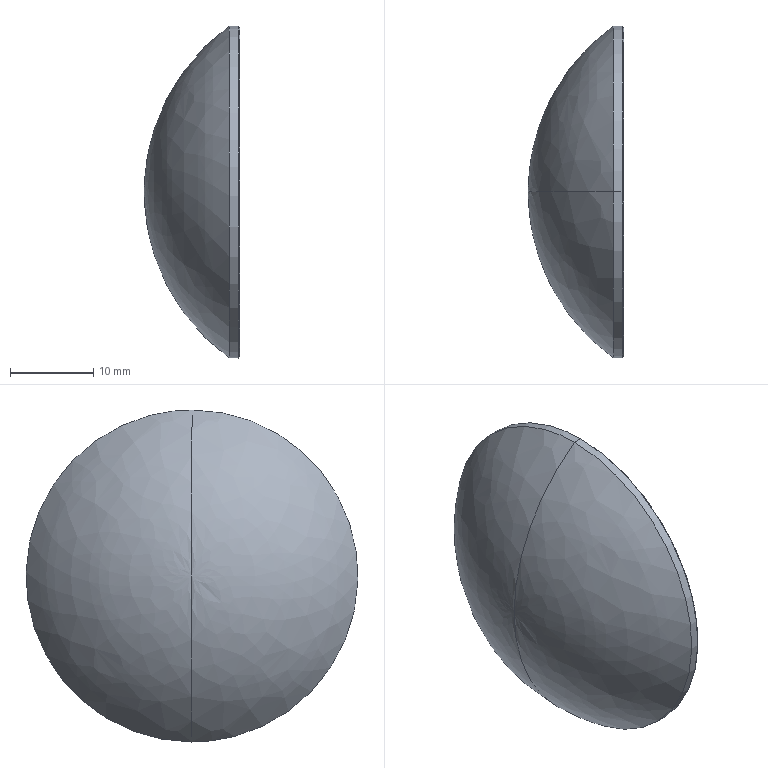Part | SolidWorks | features BaseBody 1 | 1 solid | 9 faces | box 11.433 x 39.8 x 39.8 mm | volume 7338 mm3 | spline 9
STEP:
#1=CARTESIAN_POINT('',(-56.988,0.,0.));
#2=VERTEX_POINT('',#1);
#3=CARTESIAN_POINT('',(-46.779,0.,19.9));
#4=VERTEX_POINT('',#3);
#5=CARTESIAN_POINT('',(-32.488,0.,0.));
#6=DIRECTION('',(0.,1.,0.));
#7=DIRECTION('',(-1.,0.,0.));
#8=AXIS2_PLACEMENT_3D('',#5,#6,#7);
#9=CIRCLE('',#8,24.5);
#10=EDGE_CURVE('',#2,#4,#9,.T.);
#11=ORIENTED_EDGE('',*,*,#10,.T.);
#12=CARTESIAN_POINT('',(-46.779,0.,-19.9));
#13=VERTEX_POINT('',#12);
#14=CARTESIAN_POINT('',(-46.779,0.,-19.9));
#15=CARTESIAN_POINT('',(-46.779,39.8,-19.9));
#16=CARTESIAN_POINT('',(-46.779,39.8,19.9));
#17=CARTESIAN_POINT('',(-46.779,0.,19.9));
#18=(BOUNDED_CURVE()B_SPLINE_CURVE(3,(#14,#15,#16,#17),.UNSPECIFIED.,.F.,.T.)B_SPLINE_CURVE_WITH_KNOTS((4,4),(0.,119.4),.UNSPECIFIED.)CURVE()GEOMETRIC_REPRESENTATION_ITEM()RATIONAL_B_SPLINE_CURVE((1.,0.3333,0.3333,1.))REPRESENTATION_ITEM(''));
#19=EDGE_CURVE('',#13,#4,#18,.T.);
#20=ORIENTED_EDGE('',*,*,#19,.F.);
#21=CARTESIAN_POINT('',(-32.488,0.,0.));
#22=DIRECTION('',(0.,-1.,0.));
#23=DIRECTION('',(-1.,0.,0.));
#24=AXIS2_PLACEMENT_3D('',#21,#22,#23);
#25=CIRCLE('',#24,24.5);
#26=EDGE_CURVE('',#2,#13,#25,.T.);
#27=ORIENTED_EDGE('',*,*,#26,.F.);
#28=EDGE_LOOP('',(#11,#20,#27));
#29=FACE_OUTER_BOUND('',#28,.T.);
#30=CARTESIAN_POINT('',(-56.988,0.,0.));
#31=CARTESIAN_POINT('',(-56.988,0.,0.));
#32=CARTESIAN_POINT('',(-56.988,0.,0.));
#33=CARTESIAN_POINT('',(-56.988,0.,0.));
#34=CARTESIAN_POINT('',(-56.988,0.,-8.047));
#35=CARTESIAN_POINT('',(-56.988,16.093,-8.047));
#36=CARTESIAN_POINT('',(-56.988,16.093,8.047));
#37=CARTESIAN_POINT('',(-56.988,0.,8.047));
#38=CARTESIAN_POINT('',(-53.315,0.,-15.206));
#39=CARTESIAN_POINT('',(-53.315,30.412,-15.206));
#40=CARTESIAN_POINT('',(-53.315,30.412,15.206));
#41=CARTESIAN_POINT('',(-53.315,0.,15.206));
#42=CARTESIAN_POINT('',(-46.779,0.,-19.9));
#43=CARTESIAN_POINT('',(-46.779,39.8,-19.9));
#44=CARTESIAN_POINT('',(-46.779,39.8,19.9));
#45=CARTESIAN_POINT('',(-46.779,0.,19.9));
#46=(BOUNDED_SURFACE()B_SPLINE_SURFACE(3,3,((#30,#31,#32,#33),(#34,#35,#36,#37),(#38,#39,#40,#41),(#42,#43,#44,#45)),.UNSPECIFIED.,.F.,.F.,.F.)B_SPLINE_SURFACE_WITH_KNOTS((4,4),(4,4),(0.,1.),(0.,1.),.UNSPECIFIED.)GEOMETRIC_REPRESENTATION_ITEM()RATIONAL_B_SPLINE_SURFACE(((1.,0.3333,0.3333,1.),(0.9265,0.3088,0.3088,0.9265),(0.9265,0.3088,0.3088,0.9265),(1.,0.3333,0.3333,1.)))REPRESENTATION_ITEM('')SURFACE());
#47=ADVANCED_FACE('',(#29),#46,.F.);
#48=ORIENTED_EDGE('',*,*,#26,.T.);
#49=CARTESIAN_POINT('',(-46.779,0.,19.9));
#50=CARTESIAN_POINT('',(-46.779,-39.8,19.9));
#51=CARTESIAN_POINT('',(-46.779,-39.8,-19.9));
#52=CARTESIAN_POINT('',(-46.779,0.,-19.9));
#53=(BOUNDED_CURVE()B_SPLINE_CURVE(3,(#49,#50,#51,#52),.UNSPECIFIED.,.F.,.F.)B_SPLINE_CURVE_WITH_KNOTS((4,4),(0.,119.4),.UNSPECIFIED.)CURVE()GEOMETRIC_REPRESENTATION_ITEM()RATIONAL_B_SPLINE_CURVE((1.,0.3333,0.3333,1.))REPRESENTATION_ITEM(''));
#54=EDGE_CURVE('',#4,#13,#53,.T.);
#55=ORIENTED_EDGE('',*,*,#54,.F.);
#56=ORIENTED_EDGE('',*,*,#10,.F.);
#57=EDGE_LOOP('',(#48,#55,#56));
#58=FACE_OUTER_BOUND('',#57,.T.);
#59=CARTESIAN_POINT('',(-56.988,0.,0.));
#60=CARTESIAN_POINT('',(-56.988,0.,0.));
#61=CARTESIAN_POINT('',(-56.988,0.,0.));
#62=CARTESIAN_POINT('',(-56.988,0.,0.));
#63=CARTESIAN_POINT('',(-56.988,0.,8.047));
#64=CARTESIAN_POINT('',(-56.988,-16.093,8.047));
#65=CARTESIAN_POINT('',(-56.988,-16.093,-8.047));
#66=CARTESIAN_POINT('',(-56.988,0.,-8.047));
#67=CARTESIAN_POINT('',(-53.315,0.,15.206));
#68=CARTESIAN_POINT('',(-53.315,-30.412,15.206));
#69=CARTESIAN_POINT('',(-53.315,-30.412,-15.206));
#70=CARTESIAN_POINT('',(-53.315,0.,-15.206));
#71=CARTESIAN_POINT('',(-46.779,0.,19.9));
#72=CARTESIAN_POINT('',(-46.779,-39.8,19.9));
#73=CARTESIAN_POINT('',(-46.779,-39.8,-19.9));
#74=CARTESIAN_POINT('',(-46.779,0.,-19.9));
#75=(BOUNDED_SURFACE()B_SPLINE_SURFACE(3,3,((#59,#60,#61,#62),(#63,#64,#65,#66),(#67,#68,#69,#70),(#71,#72,#73,#74)),.UNSPECIFIED.,.F.,.F.,.F.)B_SPLINE_SURFACE_WITH_KNOTS((4,4),(4,4),(0.,1.),(0.,1.),.UNSPECIFIED.)GEOMETRIC_REPRESENTATION_ITEM()RATIONAL_B_SPLINE_SURFACE(((1.,0.3333,0.3333,1.),(0.9265,0.3088,0.3088,0.9265),(0.9265,0.3088,0.3088,0.9265),(1.,0.3333,0.3333,1.)))REPRESENTATION_ITEM('')SURFACE());
#76=ADVANCED_FACE('',(#58),#75,.F.);
#77=CARTESIAN_POINT('',(-45.755,0.,19.9));
#78=VERTEX_POINT('',#77);
#79=CARTESIAN_POINT('',(-46.779,0.,19.9));
#80=DIRECTION('',(1.,0.,0.));
#81=VECTOR('',#80,1000.);
#82=LINE('',#79,#81);
#83=EDGE_CURVE('',#4,#78,#82,.T.);
#84=ORIENTED_EDGE('',*,*,#83,.F.);
#85=ORIENTED_EDGE('',*,*,#54,.T.);
#86=CARTESIAN_POINT('',(-45.755,0.,-19.9));
#87=VERTEX_POINT('',#86);
#88=CARTESIAN_POINT('',(-46.779,0.,-19.9));
#89=DIRECTION('',(1.,0.,0.));
#90=VECTOR('',#89,1000.);
#91=LINE('',#88,#90);
#92=EDGE_CURVE('',#13,#87,#91,.T.);
#93=ORIENTED_EDGE('',*,*,#92,.T.);
#94=CARTESIAN_POINT('',(-45.755,0.,19.9));
#95=CARTESIAN_POINT('',(-45.755,-39.8,19.9));
#96=CARTESIAN_POINT('',(-45.755,-39.8,-19.9));
#97=CARTESIAN_POINT('',(-45.755,0.,-19.9));
#98=(BOUNDED_CURVE()B_SPLINE_CURVE(3,(#94,#95,#96,#97),.UNSPECIFIED.,.F.,.F.)B_SPLINE_CURVE_WITH_KNOTS((4,4),(0.,119.4),.UNSPECIFIED.)CURVE()GEOMETRIC_REPRESENTATION_ITEM()RATIONAL_B_SPLINE_CURVE((1.,0.3333,0.3333,1.))REPRESENTATION_ITEM(''));
#99=EDGE_CURVE('',#78,#87,#98,.T.);
#100=ORIENTED_EDGE('',*,*,#99,.F.);
#101=EDGE_LOOP('',(#84,#85,#93,#100));
#102=FACE_OUTER_BOUND('',#101,.T.);
#103=CARTESIAN_POINT('',(-46.779,0.,19.9));
#104=CARTESIAN_POINT('',(-46.779,-39.8,19.9));
#105=CARTESIAN_POINT('',(-46.779,-39.8,-19.9));
#106=CARTESIAN_POINT('',(-46.779,0.,-19.9));
#107=CARTESIAN_POINT('',(-45.755,0.,19.9));
#108=CARTESIAN_POINT('',(-45.755,-39.8,19.9));
#109=CARTESIAN_POINT('',(-45.755,-39.8,-19.9));
#110=CARTESIAN_POINT('',(-45.755,0.,-19.9));
#111=(BOUNDED_SURFACE()B_SPLINE_SURFACE(1,3,((#103,#104,#105,#106),(#107,#108,#109,#110)),.UNSPECIFIED.,.F.,.F.,.F.)B_SPLINE_SURFACE_WITH_KNOTS((2,2),(4,4),(0.,1.024),(0.,119.4),.UNSPECIFIED.)GEOMETRIC_REPRESENTATION_ITEM()RATIONAL_B_SPLINE_SURFACE(((1.,0.3333,0.3333,1.),(1.,0.3333,0.3333,1.)))REPRESENTATION_ITEM('')SURFACE());
#112=ADVANCED_FACE('',(#102),#111,.F.);
#113=CARTESIAN_POINT('',(-45.555,0.,-19.7));
#114=VERTEX_POINT('',#113);
#115=CARTESIAN_POINT('',(-45.555,0.,-19.7));
#116=DIRECTION('',(-0.7071,0.,-0.7071));
#117=VECTOR('',#116,1000.);
#118=LINE('',#115,#117);
#119=EDGE_CURVE('',#114,#87,#118,.T.);
#120=ORIENTED_EDGE('',*,*,#119,.F.);
#121=CARTESIAN_POINT('',(-45.555,0.,19.7));
#122=VERTEX_POINT('',#121);
#123=CARTESIAN_POINT('',(-45.555,0.,19.7));
#124=CARTESIAN_POINT('',(-45.555,-2.579,19.701));
#125=CARTESIAN_POINT('',(-45.555,-5.156,19.187));
#126=CARTESIAN_POINT('',(-45.555,-8.73,17.707));
#127=CARTESIAN_POINT('',(-45.555,-9.873,17.096));
#128=CARTESIAN_POINT('',(-45.555,-12.017,15.664));
#129=CARTESIAN_POINT('',(-45.555,-13.018,14.842));
#130=CARTESIAN_POINT('',(-45.555,-14.842,13.018));
#131=CARTESIAN_POINT('',(-45.555,-15.664,12.017));
#132=CARTESIAN_POINT('',(-45.555,-17.096,9.873));
#133=CARTESIAN_POINT('',(-45.555,-17.707,8.73));
#134=CARTESIAN_POINT('',(-45.555,-18.694,6.348));
#135=CARTESIAN_POINT('',(-45.555,-19.07,5.108));
#136=CARTESIAN_POINT('',(-45.555,-19.573,2.579));
#137=CARTESIAN_POINT('',(-45.555,-19.7,1.289));
#138=CARTESIAN_POINT('',(-45.555,-19.7,-1.289));
#139=CARTESIAN_POINT('',(-45.555,-19.573,-2.579));
#140=CARTESIAN_POINT('',(-45.555,-19.07,-5.108));
#141=CARTESIAN_POINT('',(-45.555,-18.694,-6.348));
#142=CARTESIAN_POINT('',(-45.555,-17.707,-8.73));
#143=CARTESIAN_POINT('',(-45.555,-17.096,-9.873));
#144=CARTESIAN_POINT('',(-45.555,-15.664,-12.017));
#145=CARTESIAN_POINT('',(-45.555,-14.842,-13.018));
#146=CARTESIAN_POINT('',(-45.555,-13.018,-14.842));
#147=CARTESIAN_POINT('',(-45.555,-12.017,-15.664));
#148=CARTESIAN_POINT('',(-45.555,-9.873,-17.096));
#149=CARTESIAN_POINT('',(-45.555,-8.73,-17.707));
#150=CARTESIAN_POINT('',(-45.555,-5.156,-19.187));
#151=CARTESIAN_POINT('',(-45.555,-2.579,-19.701));
#152=CARTESIAN_POINT('',(-45.555,0.,-19.7));
#153=B_SPLINE_CURVE_WITH_KNOTS('',3,(#123,#124,#125,#126,#127,#128,#129,#130,#131,#132,#133,#134,#135,#136,#137,#138,#139,#140,#141,#142,#143,#144,#145,#146,#147,#148,#149,#150,#151,#152),.UNSPECIFIED.,.F.,.F.,(4,2,2,2,2,2,2,2,2,2,2,2,2,2,4),(0.,0.125,0.1875,0.25,0.3125,0.375,0.4375,0.5,0.5625,0.625,0.6875,0.75,0.8125,0.875,1.),.UNSPECIFIED.);
#154=EDGE_CURVE('',#122,#114,#153,.T.);
#155=ORIENTED_EDGE('',*,*,#154,.F.);
#156=CARTESIAN_POINT('',(-45.555,0.,19.7));
#157=DIRECTION('',(-0.7071,0.,0.7071));
#158=VECTOR('',#157,1000.);
#159=LINE('',#156,#158);
#160=EDGE_CURVE('',#122,#78,#159,.T.);
#161=ORIENTED_EDGE('',*,*,#160,.T.);
#162=ORIENTED_EDGE('',*,*,#99,.T.);
#163=EDGE_LOOP('',(#120,#155,#161,#162));
#164=FACE_OUTER_BOUND('',#163,.T.);
#165=CARTESIAN_POINT('',(-45.555,0.,-19.7));
#166=CARTESIAN_POINT('',(-45.555,-39.399,-19.7));
#167=CARTESIAN_POINT('',(-45.555,-39.399,19.7));
#168=CARTESIAN_POINT('',(-45.555,0.,19.7));
#169=CARTESIAN_POINT('',(-45.755,0.,-19.9));
#170=CARTESIAN_POINT('',(-45.755,-39.8,-19.9));
#171=CARTESIAN_POINT('',(-45.755,-39.8,19.9));
#172=CARTESIAN_POINT('',(-45.755,0.,19.9));
#173=(BOUNDED_SURFACE()B_SPLINE_SURFACE(1,3,((#165,#166,#167,#168),(#169,#170,#171,#172)),.UNSPECIFIED.,.F.,.F.,.F.)B_SPLINE_SURFACE_WITH_KNOTS((2,2),(4,4),(-0.001621,1.),(0.,119.4),.UNSPECIFIED.)GEOMETRIC_REPRESENTATION_ITEM()RATIONAL_B_SPLINE_SURFACE(((1.,0.3333,0.3333,1.),(1.,0.3333,0.3333,1.)))REPRESENTATION_ITEM('')SURFACE());
#174=ADVANCED_FACE('',(#164),#173,.F.);
#175=CARTESIAN_POINT('',(-45.555,0.,-19.7));
#176=CARTESIAN_POINT('',(-45.555,2.579,-19.701));
#177=CARTESIAN_POINT('',(-45.555,5.156,-19.187));
#178=CARTESIAN_POINT('',(-45.555,8.73,-17.707));
#179=CARTESIAN_POINT('',(-45.555,9.873,-17.096));
#180=CARTESIAN_POINT('',(-45.555,12.017,-15.664));
#181=CARTESIAN_POINT('',(-45.555,13.018,-14.842));
#182=CARTESIAN_POINT('',(-45.555,14.842,-13.018));
#183=CARTESIAN_POINT('',(-45.555,15.664,-12.017));
#184=CARTESIAN_POINT('',(-45.555,17.096,-9.873));
#185=CARTESIAN_POINT('',(-45.555,17.707,-8.73));
#186=CARTESIAN_POINT('',(-45.555,18.694,-6.348));
#187=CARTESIAN_POINT('',(-45.555,19.07,-5.108));
#188=CARTESIAN_POINT('',(-45.555,19.573,-2.579));
#189=CARTESIAN_POINT('',(-45.555,19.7,-1.289));
#190=CARTESIAN_POINT('',(-45.555,19.7,1.289));
#191=CARTESIAN_POINT('',(-45.555,19.573,2.579));
#192=CARTESIAN_POINT('',(-45.555,19.07,5.108));
#193=CARTESIAN_POINT('',(-45.555,18.694,6.348));
#194=CARTESIAN_POINT('',(-45.555,17.707,8.73));
#195=CARTESIAN_POINT('',(-45.555,17.096,9.873));
#196=CARTESIAN_POINT('',(-45.555,15.664,12.017));
#197=CARTESIAN_POINT('',(-45.555,14.842,13.018));
#198=CARTESIAN_POINT('',(-45.555,13.018,14.842));
#199=CARTESIAN_POINT('',(-45.555,12.017,15.664));
#200=CARTESIAN_POINT('',(-45.555,9.873,17.096));
#201=CARTESIAN_POINT('',(-45.555,8.73,17.707));
#202=CARTESIAN_POINT('',(-45.555,5.156,19.187));
#203=CARTESIAN_POINT('',(-45.555,2.579,19.701));
#204=CARTESIAN_POINT('',(-45.555,0.,19.7));
#205=B_SPLINE_CURVE_WITH_KNOTS('',3,(#175,#176,#177,#178,#179,#180,#181,#182,#183,#184,#185,#186,#187,#188,#189,#190,#191,#192,#193,#194,#195,#196,#197,#198,#199,#200,#201,#202,#203,#204),.UNSPECIFIED.,.F.,.F.,(4,2,2,2,2,2,2,2,2,2,2,2,2,2,4),(0.,0.125,0.1875,0.25,0.3125,0.375,0.4375,0.5,0.5625,0.625,0.6875,0.75,0.8125,0.875,1.),.UNSPECIFIED.);
#206=EDGE_CURVE('',#114,#122,#205,.T.);
#207=ORIENTED_EDGE('',*,*,#206,.F.);
#208=ORIENTED_EDGE('',*,*,#119,.T.);
#209=CARTESIAN_POINT('',(-45.755,0.,-19.9));
#210=CARTESIAN_POINT('',(-45.755,39.8,-19.9));
#211=CARTESIAN_POINT('',(-45.755,39.8,19.9));
#212=CARTESIAN_POINT('',(-45.755,0.,19.9));
#213=(BOUNDED_CURVE()B_SPLINE_CURVE(3,(#209,#210,#211,#212),.UNSPECIFIED.,.F.,.T.)B_SPLINE_CURVE_WITH_KNOTS((4,4),(0.,119.4),.UNSPECIFIED.)CURVE()GEOMETRIC_REPRESENTATION_ITEM()RATIONAL_B_SPLINE_CURVE((1.,0.3333,0.3333,1.))REPRESENTATION_ITEM(''));
#214=EDGE_CURVE('',#87,#78,#213,.T.);
#215=ORIENTED_EDGE('',*,*,#214,.T.);
#216=ORIENTED_EDGE('',*,*,#160,.F.);
#217=EDGE_LOOP('',(#207,#208,#215,#216));
#218=FACE_OUTER_BOUND('',#217,.T.);
#219=CARTESIAN_POINT('',(-45.555,0.,19.7));
#220=CARTESIAN_POINT('',(-45.555,39.399,19.7));
#221=CARTESIAN_POINT('',(-45.555,39.399,-19.7));
#222=CARTESIAN_POINT('',(-45.555,0.,-19.7));
#223=CARTESIAN_POINT('',(-45.755,0.,19.9));
#224=CARTESIAN_POINT('',(-45.755,39.8,19.9));
#225=CARTESIAN_POINT('',(-45.755,39.8,-19.9));
#226=CARTESIAN_POINT('',(-45.755,0.,-19.9));
#227=(BOUNDED_SURFACE()B_SPLINE_SURFACE(1,3,((#219,#220,#221,#222),(#223,#224,#225,#226)),.UNSPECIFIED.,.F.,.F.,.F.)B_SPLINE_SURFACE_WITH_KNOTS((2,2),(4,4),(-0.001621,1.),(0.,119.4),.UNSPECIFIED.)GEOMETRIC_REPRESENTATION_ITEM()RATIONAL_B_SPLINE_SURFACE(((1.,0.3333,0.3333,1.),(1.,0.3333,0.3333,1.)))REPRESENTATION_ITEM('')SURFACE());
#228=ADVANCED_FACE('',(#218),#227,.F.);
#229=ORIENTED_EDGE('',*,*,#19,.T.);
#230=ORIENTED_EDGE('',*,*,#83,.T.);
#231=ORIENTED_EDGE('',*,*,#214,.F.);
#232=ORIENTED_EDGE('',*,*,#92,.F.);
#233=EDGE_LOOP('',(#229,#230,#231,#232));
#234=FACE_OUTER_BOUND('',#233,.T.);
#235=CARTESIAN_POINT('',(-46.779,0.,-19.9));
#236=CARTESIAN_POINT('',(-46.779,39.8,-19.9));
#237=CARTESIAN_POINT('',(-46.779,39.8,19.9));
#238=CARTESIAN_POINT('',(-46.779,0.,19.9));
#239=CARTESIAN_POINT('',(-45.755,0.,-19.9));
#240=CARTESIAN_POINT('',(-45.755,39.8,-19.9));
#241=CARTESIAN_POINT('',(-45.755,39.8,19.9));
#242=CARTESIAN_POINT('',(-45.755,0.,19.9));
#243=(BOUNDED_SURFACE()B_SPLINE_SURFACE(1,3,((#235,#236,#237,#238),(#239,#240,#241,#242)),.UNSPECIFIED.,.F.,.F.,.F.)B_SPLINE_SURFACE_WITH_KNOTS((2,2),(4,4),(0.,1.024),(0.,119.4),.UNSPECIFIED.)GEOMETRIC_REPRESENTATION_ITEM()RATIONAL_B_SPLINE_SURFACE(((1.,0.3333,0.3333,1.),(1.,0.3333,0.3333,1.)))REPRESENTATION_ITEM('')SURFACE());
#244=ADVANCED_FACE('',(#234),#243,.F.);
#245=CARTESIAN_POINT('',(-45.555,0.,-17.659));
#246=VERTEX_POINT('',#245);
#247=CARTESIAN_POINT('',(-45.555,0.,17.659));
#248=VERTEX_POINT('',#247);
#249=CARTESIAN_POINT('',(-45.555,0.,-17.659));
#250=CARTESIAN_POINT('',(-45.555,-2.312,-17.66));
#251=CARTESIAN_POINT('',(-45.555,-4.622,-17.199));
#252=CARTESIAN_POINT('',(-45.555,-7.826,-15.873));
#253=CARTESIAN_POINT('',(-45.555,-8.85,-15.325));
#254=CARTESIAN_POINT('',(-45.555,-10.772,-14.041));
#255=CARTESIAN_POINT('',(-45.555,-11.67,-13.304));
#256=CARTESIAN_POINT('',(-45.555,-13.304,-11.67));
#257=CARTESIAN_POINT('',(-45.555,-14.041,-10.772));
#258=CARTESIAN_POINT('',(-45.555,-15.325,-8.85));
#259=CARTESIAN_POINT('',(-45.555,-15.873,-7.826));
#260=CARTESIAN_POINT('',(-45.555,-16.757,-5.69));
#261=CARTESIAN_POINT('',(-45.555,-17.094,-4.579));
#262=CARTESIAN_POINT('',(-45.555,-17.545,-2.312));
#263=CARTESIAN_POINT('',(-45.555,-17.659,-1.156));
#264=CARTESIAN_POINT('',(-45.555,-17.659,1.156));
#265=CARTESIAN_POINT('',(-45.555,-17.545,2.312));
#266=CARTESIAN_POINT('',(-45.555,-17.094,4.579));
#267=CARTESIAN_POINT('',(-45.555,-16.757,5.69));
#268=CARTESIAN_POINT('',(-45.555,-15.873,7.826));
#269=CARTESIAN_POINT('',(-45.555,-15.325,8.85));
#270=CARTESIAN_POINT('',(-45.555,-14.041,10.772));
#271=CARTESIAN_POINT('',(-45.555,-13.304,11.67));
#272=CARTESIAN_POINT('',(-45.555,-11.67,13.304));
#273=CARTESIAN_POINT('',(-45.555,-10.772,14.041));
#274=CARTESIAN_POINT('',(-45.555,-8.85,15.325));
#275=CARTESIAN_POINT('',(-45.555,-7.826,15.872));
#276=CARTESIAN_POINT('',(-45.555,-4.622,17.199));
#277=CARTESIAN_POINT('',(-45.555,-2.312,17.66));
#278=CARTESIAN_POINT('',(-45.555,0.,17.659));
#279=B_SPLINE_CURVE_WITH_KNOTS('',3,(#249,#250,#251,#252,#253,#254,#255,#256,#257,#258,#259,#260,#261,#262,#263,#264,#265,#266,#267,#268,#269,#270,#271,#272,#273,#274,#275,#276,#277,#278),.UNSPECIFIED.,.F.,.F.,(4,2,2,2,2,2,2,2,2,2,2,2,2,2,4),(0.,0.125,0.1875,0.25,0.3125,0.375,0.4375,0.5,0.5625,0.625,0.6875,0.75,0.8125,0.875,1.),.UNSPECIFIED.);
#280=EDGE_CURVE('',#246,#248,#279,.T.);
#281=ORIENTED_EDGE('',*,*,#280,.T.);
#282=CARTESIAN_POINT('',(-45.555,0.,17.659));
#283=CARTESIAN_POINT('',(-45.555,2.312,17.66));
#284=CARTESIAN_POINT('',(-45.555,4.622,17.199));
#285=CARTESIAN_POINT('',(-45.555,7.826,15.873));
#286=CARTESIAN_POINT('',(-45.555,8.85,15.325));
#287=CARTESIAN_POINT('',(-45.555,10.772,14.041));
#288=CARTESIAN_POINT('',(-45.555,11.67,13.304));
#289=CARTESIAN_POINT('',(-45.555,13.304,11.67));
#290=CARTESIAN_POINT('',(-45.555,14.041,10.772));
#291=CARTESIAN_POINT('',(-45.555,15.325,8.85));
#292=CARTESIAN_POINT('',(-45.555,15.873,7.826));
#293=CARTESIAN_POINT('',(-45.555,16.757,5.69));
#294=CARTESIAN_POINT('',(-45.555,17.094,4.579));
#295=CARTESIAN_POINT('',(-45.555,17.545,2.312));
#296=CARTESIAN_POINT('',(-45.555,17.659,1.156));
#297=CARTESIAN_POINT('',(-45.555,17.659,-1.156));
#298=CARTESIAN_POINT('',(-45.555,17.545,-2.312));
#299=CARTESIAN_POINT('',(-45.555,17.094,-4.579));
#300=CARTESIAN_POINT('',(-45.555,16.757,-5.69));
#301=CARTESIAN_POINT('',(-45.555,15.873,-7.826));
#302=CARTESIAN_POINT('',(-45.555,15.325,-8.85));
#303=CARTESIAN_POINT('',(-45.555,14.041,-10.772));
#304=CARTESIAN_POINT('',(-45.555,13.304,-11.67));
#305=CARTESIAN_POINT('',(-45.555,11.67,-13.304));
#306=CARTESIAN_POINT('',(-45.555,10.772,-14.041));
#307=CARTESIAN_POINT('',(-45.555,8.85,-15.325));
#308=CARTESIAN_POINT('',(-45.555,7.826,-15.872));
#309=CARTESIAN_POINT('',(-45.555,4.622,-17.199));
#310=CARTESIAN_POINT('',(-45.555,2.312,-17.66));
#311=CARTESIAN_POINT('',(-45.555,0.,-17.659));
#312=B_SPLINE_CURVE_WITH_KNOTS('',3,(#282,#283,#284,#285,#286,#287,#288,#289,#290,#291,#292,#293,#294,#295,#296,#297,#298,#299,#300,#301,#302,#303,#304,#305,#306,#307,#308,#309,#310,#311),.UNSPECIFIED.,.F.,.F.,(4,2,2,2,2,2,2,2,2,2,2,2,2,2,4),(0.,0.125,0.1875,0.25,0.3125,0.375,0.4375,0.5,0.5625,0.625,0.6875,0.75,0.8125,0.875,1.),.UNSPECIFIED.);
#313=EDGE_CURVE('',#248,#246,#312,.T.);
#314=ORIENTED_EDGE('',*,*,#313,.T.);
#315=EDGE_LOOP('',(#281,#314));
#316=FACE_BOUND('',#315,.T.);
#317=ORIENTED_EDGE('',*,*,#206,.T.);
#318=ORIENTED_EDGE('',*,*,#154,.T.);
#319=EDGE_LOOP('',(#317,#318));
#320=FACE_OUTER_BOUND('',#319,.T.);
#321=CARTESIAN_POINT('',(-45.555,-19.897,19.897));
#322=CARTESIAN_POINT('',(-45.555,19.897,19.897));
#323=CARTESIAN_POINT('',(-45.555,-19.897,-19.897));
#324=CARTESIAN_POINT('',(-45.555,19.897,-19.897));
#325=B_SPLINE_SURFACE_WITH_KNOTS('',1,1,((#321,#322),(#323,#324)),.UNSPECIFIED.,.F.,.F.,.F.,(2,2),(2,2),(-19.897,19.897),(-19.897,19.897),.UNSPECIFIED.);
#326=ADVANCED_FACE('',(#316,#320),#325,.T.);
#327=CARTESIAN_POINT('',(-47.77,0.,0.));
#328=VERTEX_POINT('',#327);
#329=CARTESIAN_POINT('',(23.729,0.,0.));
#330=DIRECTION('',(0.,-1.,0.));
#331=DIRECTION('',(-1.,0.,0.));
#332=AXIS2_PLACEMENT_3D('',#329,#330,#331);
#333=CIRCLE('',#332,71.499);
#334=EDGE_CURVE('',#328,#246,#333,.T.);
#335=ORIENTED_EDGE('',*,*,#334,.T.);
#336=ORIENTED_EDGE('',*,*,#313,.F.);
#337=CARTESIAN_POINT('',(23.729,0.,0.));
#338=DIRECTION('',(0.,1.,0.));
#339=DIRECTION('',(-1.,0.,0.));
#340=AXIS2_PLACEMENT_3D('',#337,#338,#339);
#341=CIRCLE('',#340,71.499);
#342=EDGE_CURVE('',#328,#248,#341,.T.);
#343=ORIENTED_EDGE('',*,*,#342,.F.);
#344=EDGE_LOOP('',(#335,#336,#343));
#345=FACE_OUTER_BOUND('',#344,.T.);
#346=CARTESIAN_POINT('',(-47.77,0.,0.));
#347=CARTESIAN_POINT('',(-47.77,0.,0.));
#348=CARTESIAN_POINT('',(-47.77,0.,0.));
#349=CARTESIAN_POINT('',(-47.77,0.,0.));
#350=CARTESIAN_POINT('',(-47.77,0.,-5.963));
#351=CARTESIAN_POINT('',(-47.77,11.927,-5.963));
#352=CARTESIAN_POINT('',(-47.77,11.927,5.963));
#353=CARTESIAN_POINT('',(-47.77,0.,5.963));
#354=CARTESIAN_POINT('',(-47.028,0.,-11.88));
#355=CARTESIAN_POINT('',(-47.028,23.761,-11.88));
#356=CARTESIAN_POINT('',(-47.028,23.761,11.88));
#357=CARTESIAN_POINT('',(-47.028,0.,11.88));
#358=CARTESIAN_POINT('',(-45.555,0.,-17.659));
#359=CARTESIAN_POINT('',(-45.555,35.318,-17.659));
#360=CARTESIAN_POINT('',(-45.555,35.318,17.659));
#361=CARTESIAN_POINT('',(-45.555,0.,17.659));
#362=(BOUNDED_SURFACE()B_SPLINE_SURFACE(3,3,((#346,#347,#348,#349),(#350,#351,#352,#353),(#354,#355,#356,#357),(#358,#359,#360,#361)),.UNSPECIFIED.,.F.,.F.,.F.)B_SPLINE_SURFACE_WITH_KNOTS((4,4),(4,4),(0.,1.),(0.,1.),.UNSPECIFIED.)GEOMETRIC_REPRESENTATION_ITEM()RATIONAL_B_SPLINE_SURFACE(((1.,0.3333,0.3333,1.),(0.9948,0.3316,0.3316,0.9948),(0.9948,0.3316,0.3316,0.9948),(1.,0.3333,0.3333,1.)))REPRESENTATION_ITEM('')SURFACE());
#363=ADVANCED_FACE('',(#345),#362,.T.);
#364=ORIENTED_EDGE('',*,*,#342,.T.);
#365=ORIENTED_EDGE('',*,*,#280,.F.);
#366=ORIENTED_EDGE('',*,*,#334,.F.);
#367=EDGE_LOOP('',(#364,#365,#366));
#368=FACE_OUTER_BOUND('',#367,.T.);
#369=CARTESIAN_POINT('',(-47.77,0.,0.));
#370=CARTESIAN_POINT('',(-47.77,0.,0.));
#371=CARTESIAN_POINT('',(-47.77,0.,0.));
#372=CARTESIAN_POINT('',(-47.77,0.,0.));
#373=CARTESIAN_POINT('',(-47.77,0.,5.963));
#374=CARTESIAN_POINT('',(-47.77,-11.927,5.963));
#375=CARTESIAN_POINT('',(-47.77,-11.927,-5.963));
#376=CARTESIAN_POINT('',(-47.77,0.,-5.963));
#377=CARTESIAN_POINT('',(-47.028,0.,11.88));
#378=CARTESIAN_POINT('',(-47.028,-23.761,11.88));
#379=CARTESIAN_POINT('',(-47.028,-23.761,-11.88));
#380=CARTESIAN_POINT('',(-47.028,0.,-11.88));
#381=CARTESIAN_POINT('',(-45.555,0.,17.659));
#382=CARTESIAN_POINT('',(-45.555,-35.318,17.659));
#383=CARTESIAN_POINT('',(-45.555,-35.318,-17.659));
#384=CARTESIAN_POINT('',(-45.555,0.,-17.659));
#385=(BOUNDED_SURFACE()B_SPLINE_SURFACE(3,3,((#369,#370,#371,#372),(#373,#374,#375,#376),(#377,#378,#379,#380),(#381,#382,#383,#384)),.UNSPECIFIED.,.F.,.F.,.T.)B_SPLINE_SURFACE_WITH_KNOTS((4,4),(4,4),(0.,1.),(0.,1.),.UNSPECIFIED.)GEOMETRIC_REPRESENTATION_ITEM()RATIONAL_B_SPLINE_SURFACE(((1.,0.3333,0.3333,1.),(0.9948,0.3316,0.3316,0.9948),(0.9948,0.3316,0.3316,0.9948),(1.,0.3333,0.3333,1.)))REPRESENTATION_ITEM('')SURFACE());
#386=ADVANCED_FACE('',(#368),#385,.T.);
#387=CLOSED_SHELL('',(#47,#76,#112,#174,#228,#244,#326,#363,#386));
#388=MANIFOLD_SOLID_BREP('',#387);
#389=CARTESIAN_POINT('',(0.,0.,0.));
#390=DIRECTION('',(0.,0.,1.));
#391=DIRECTION('',(1.,0.,0.));
#392=AXIS2_PLACEMENT_3D('',#389,#390,#391);
#393=(LENGTH_UNIT()NAMED_UNIT(*)SI_UNIT(.MILLI.,.METRE.));
#394=UNCERTAINTY_MEASURE_WITH_UNIT(LENGTH_MEASURE(0.00001),#393,'','');
#395=(NAMED_UNIT(*)PLANE_ANGLE_UNIT()SI_UNIT($,.RADIAN.));
#396=(NAMED_UNIT(*)SI_UNIT($,.STERADIAN.)SOLID_ANGLE_UNIT());
#397=(GEOMETRIC_REPRESENTATION_CONTEXT(3)GLOBAL_UNCERTAINTY_ASSIGNED_CONTEXT((#394))GLOBAL_UNIT_ASSIGNED_CONTEXT((#393,#395,#396))REPRESENTATION_CONTEXT('',''));
#398=ADVANCED_BREP_SHAPE_REPRESENTATION('',(#388,#392),#397);